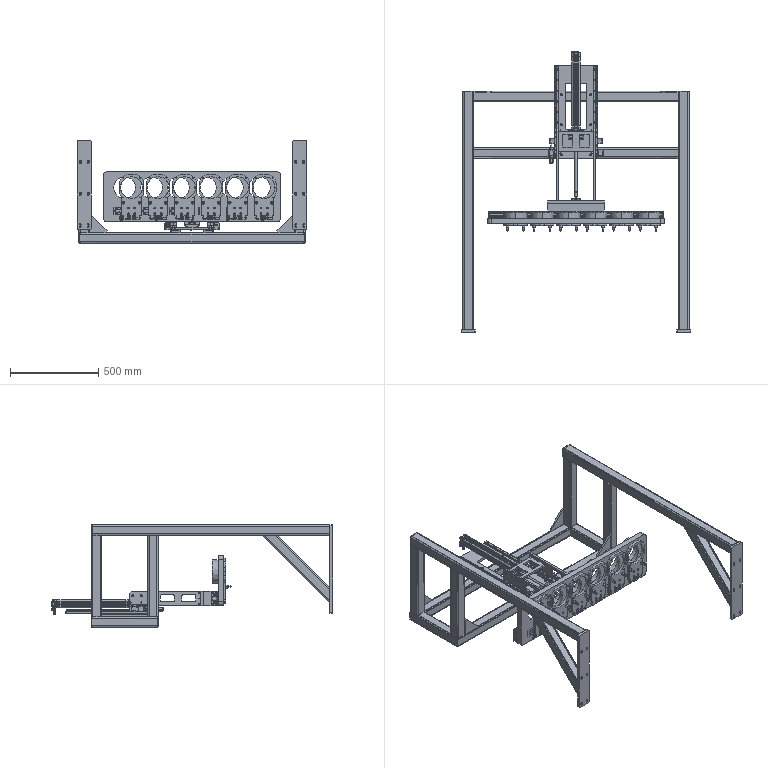Part | SolidWorks | 122 solids | 4797 faces | volume 24248419 mm3 | plane 2220 | cylinder 1954 | cone 576 | sphere 24 | torus 12 | spline 11 | commonest cylinder face diameters 5.5 x168 10 x168 8 x132 11 x114 5 x112 4.2 x108